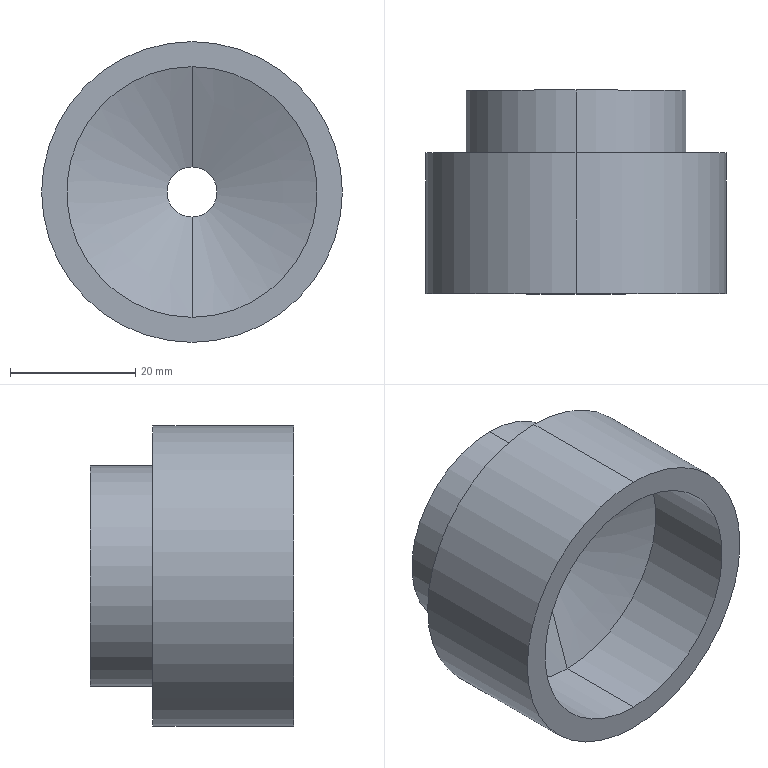Part | SolidWorks | features Revolution 1 | 1 solid | 13 faces | box 48 x 32.5 x 48 mm | volume 28090 mm3 | cylinder 8 | plane 3 | cone 2 | commonest cylinder face diameters 8 x2 35.2 x2 40 x2 48 x2
STEP:
#1=CARTESIAN_POINT('',(0.,0.,24.));
#2=VERTEX_POINT('',#1);
#3=CARTESIAN_POINT('',(0.,0.,-24.));
#4=VERTEX_POINT('',#3);
#5=CARTESIAN_POINT('',(0.,0.,0.));
#6=DIRECTION('',(0.,1.,0.));
#7=DIRECTION('',(0.,0.,1.));
#8=AXIS2_PLACEMENT_3D('',#5,#6,#7);
#9=CIRCLE('',#8,24.);
#10=EDGE_CURVE('',#2,#4,#9,.T.);
#11=ORIENTED_EDGE('',*,*,#10,.T.);
#12=CARTESIAN_POINT('',(0.,22.5,-24.));
#13=VERTEX_POINT('',#12);
#14=CARTESIAN_POINT('',(0.,61.8,-24.));
#15=DIRECTION('',(0.,1.,0.));
#16=VECTOR('',#15,1000.);
#17=LINE('',#14,#16);
#18=EDGE_CURVE('',#4,#13,#17,.T.);
#19=ORIENTED_EDGE('',*,*,#18,.T.);
#20=CARTESIAN_POINT('',(0.,22.5,24.));
#21=VERTEX_POINT('',#20);
#22=CARTESIAN_POINT('',(0.,22.5,0.));
#23=DIRECTION('',(0.,1.,0.));
#24=DIRECTION('',(0.,0.,1.));
#25=AXIS2_PLACEMENT_3D('',#22,#23,#24);
#26=CIRCLE('',#25,24.);
#27=EDGE_CURVE('',#21,#13,#26,.T.);
#28=ORIENTED_EDGE('',*,*,#27,.F.);
#29=CARTESIAN_POINT('',(0.,61.8,24.));
#30=DIRECTION('',(0.,1.,0.));
#31=VECTOR('',#30,1000.);
#32=LINE('',#29,#31);
#33=EDGE_CURVE('',#2,#21,#32,.T.);
#34=ORIENTED_EDGE('',*,*,#33,.F.);
#35=EDGE_LOOP('',(#11,#19,#28,#34));
#36=FACE_OUTER_BOUND('',#35,.T.);
#37=CARTESIAN_POINT('',(0.,61.8,0.));
#38=DIRECTION('',(0.,1.,0.));
#39=DIRECTION('',(0.,0.,1.));
#40=AXIS2_PLACEMENT_3D('',#37,#38,#39);
#41=CYLINDRICAL_SURFACE('',#40,24.);
#42=ADVANCED_FACE('',(#36),#41,.T.);
#43=CARTESIAN_POINT('',(0.,22.5,17.6));
#44=VERTEX_POINT('',#43);
#45=CARTESIAN_POINT('',(0.,22.5,-17.6));
#46=VERTEX_POINT('',#45);
#47=CARTESIAN_POINT('',(0.,22.5,0.));
#48=DIRECTION('',(0.,1.,0.));
#49=DIRECTION('',(0.,0.,1.));
#50=AXIS2_PLACEMENT_3D('',#47,#48,#49);
#51=CIRCLE('',#50,17.6);
#52=EDGE_CURVE('',#44,#46,#51,.T.);
#53=ORIENTED_EDGE('',*,*,#52,.T.);
#54=CARTESIAN_POINT('',(0.,32.5,-17.6));
#55=VERTEX_POINT('',#54);
#56=CARTESIAN_POINT('',(0.,61.8,-17.6));
#57=DIRECTION('',(0.,1.,0.));
#58=VECTOR('',#57,1000.);
#59=LINE('',#56,#58);
#60=EDGE_CURVE('',#46,#55,#59,.T.);
#61=ORIENTED_EDGE('',*,*,#60,.T.);
#62=CARTESIAN_POINT('',(0.,32.5,17.6));
#63=VERTEX_POINT('',#62);
#64=CARTESIAN_POINT('',(0.,32.5,0.));
#65=DIRECTION('',(0.,1.,0.));
#66=DIRECTION('',(0.,0.,1.));
#67=AXIS2_PLACEMENT_3D('',#64,#65,#66);
#68=CIRCLE('',#67,17.6);
#69=EDGE_CURVE('',#63,#55,#68,.T.);
#70=ORIENTED_EDGE('',*,*,#69,.F.);
#71=CARTESIAN_POINT('',(0.,61.8,17.6));
#72=DIRECTION('',(0.,1.,0.));
#73=VECTOR('',#72,1000.);
#74=LINE('',#71,#73);
#75=EDGE_CURVE('',#44,#63,#74,.T.);
#76=ORIENTED_EDGE('',*,*,#75,.F.);
#77=EDGE_LOOP('',(#53,#61,#70,#76));
#78=FACE_OUTER_BOUND('',#77,.T.);
#79=CARTESIAN_POINT('',(0.,61.8,0.));
#80=DIRECTION('',(0.,1.,0.));
#81=DIRECTION('',(0.,0.,1.));
#82=AXIS2_PLACEMENT_3D('',#79,#80,#81);
#83=CYLINDRICAL_SURFACE('',#82,17.6);
#84=ADVANCED_FACE('',(#78),#83,.T.);
#85=CARTESIAN_POINT('',(0.,20.6,-4.));
#86=VERTEX_POINT('',#85);
#87=CARTESIAN_POINT('',(0.,20.6,4.));
#88=VERTEX_POINT('',#87);
#89=CARTESIAN_POINT('',(0.,20.6,0.));
#90=DIRECTION('',(0.,1.,0.));
#91=DIRECTION('',(0.,0.,1.));
#92=AXIS2_PLACEMENT_3D('',#89,#90,#91);
#93=CIRCLE('',#92,4.);
#94=EDGE_CURVE('',#86,#88,#93,.T.);
#95=ORIENTED_EDGE('',*,*,#94,.F.);
#96=CARTESIAN_POINT('',(0.,32.5,-4.));
#97=VERTEX_POINT('',#96);
#98=CARTESIAN_POINT('',(0.,61.8,-4.));
#99=DIRECTION('',(0.,1.,0.));
#100=VECTOR('',#99,1000.);
#101=LINE('',#98,#100);
#102=EDGE_CURVE('',#86,#97,#101,.T.);
#103=ORIENTED_EDGE('',*,*,#102,.T.);
#104=CARTESIAN_POINT('',(0.,32.5,4.));
#105=VERTEX_POINT('',#104);
#106=CARTESIAN_POINT('',(0.,32.5,0.));
#107=DIRECTION('',(0.,1.,0.));
#108=DIRECTION('',(0.,0.,1.));
#109=AXIS2_PLACEMENT_3D('',#106,#107,#108);
#110=CIRCLE('',#109,4.);
#111=EDGE_CURVE('',#97,#105,#110,.T.);
#112=ORIENTED_EDGE('',*,*,#111,.T.);
#113=CARTESIAN_POINT('',(0.,61.8,4.));
#114=DIRECTION('',(0.,1.,0.));
#115=VECTOR('',#114,1000.);
#116=LINE('',#113,#115);
#117=EDGE_CURVE('',#88,#105,#116,.T.);
#118=ORIENTED_EDGE('',*,*,#117,.F.);
#119=EDGE_LOOP('',(#95,#103,#112,#118));
#120=FACE_OUTER_BOUND('',#119,.T.);
#121=CARTESIAN_POINT('',(0.,61.8,0.));
#122=DIRECTION('',(0.,1.,0.));
#123=DIRECTION('',(0.,0.,1.));
#124=AXIS2_PLACEMENT_3D('',#121,#122,#123);
#125=CYLINDRICAL_SURFACE('',#124,4.);
#126=ADVANCED_FACE('',(#120),#125,.F.);
#127=ORIENTED_EDGE('',*,*,#94,.T.);
#128=CARTESIAN_POINT('',(0.,15.,20.));
#129=VERTEX_POINT('',#128);
#130=CARTESIAN_POINT('',(0.,15.,20.));
#131=DIRECTION('',(0.,-0.3304,0.9439));
#132=VECTOR('',#131,1000.);
#133=LINE('',#130,#132);
#134=EDGE_CURVE('',#88,#129,#133,.T.);
#135=ORIENTED_EDGE('',*,*,#134,.T.);
#136=CARTESIAN_POINT('',(0.,15.,-20.));
#137=VERTEX_POINT('',#136);
#138=CARTESIAN_POINT('',(0.,15.,0.));
#139=DIRECTION('',(0.,1.,0.));
#140=DIRECTION('',(0.,0.,1.));
#141=AXIS2_PLACEMENT_3D('',#138,#139,#140);
#142=CIRCLE('',#141,20.);
#143=EDGE_CURVE('',#137,#129,#142,.T.);
#144=ORIENTED_EDGE('',*,*,#143,.F.);
#145=CARTESIAN_POINT('',(0.,15.,-20.));
#146=DIRECTION('',(0.,-0.3304,-0.9439));
#147=VECTOR('',#146,1000.);
#148=LINE('',#145,#147);
#149=EDGE_CURVE('',#86,#137,#148,.T.);
#150=ORIENTED_EDGE('',*,*,#149,.F.);
#151=EDGE_LOOP('',(#127,#135,#144,#150));
#152=FACE_OUTER_BOUND('',#151,.T.);
#153=CARTESIAN_POINT('',(0.,15.,0.));
#154=DIRECTION('',(0.,-1.,0.));
#155=DIRECTION('',(0.,0.,-1.));
#156=AXIS2_PLACEMENT_3D('',#153,#154,#155);
#157=CONICAL_SURFACE('',#156,20.,1.234);
#158=ADVANCED_FACE('',(#152),#157,.F.);
#159=CARTESIAN_POINT('',(0.,0.,-20.));
#160=VERTEX_POINT('',#159);
#161=CARTESIAN_POINT('',(0.,0.,20.));
#162=VERTEX_POINT('',#161);
#163=CARTESIAN_POINT('',(0.,0.,0.));
#164=DIRECTION('',(0.,1.,0.));
#165=DIRECTION('',(0.,0.,1.));
#166=AXIS2_PLACEMENT_3D('',#163,#164,#165);
#167=CIRCLE('',#166,20.);
#168=EDGE_CURVE('',#160,#162,#167,.T.);
#169=ORIENTED_EDGE('',*,*,#168,.F.);
#170=CARTESIAN_POINT('',(0.,61.8,-20.));
#171=DIRECTION('',(0.,1.,0.));
#172=VECTOR('',#171,1000.);
#173=LINE('',#170,#172);
#174=EDGE_CURVE('',#160,#137,#173,.T.);
#175=ORIENTED_EDGE('',*,*,#174,.T.);
#176=ORIENTED_EDGE('',*,*,#143,.T.);
#177=CARTESIAN_POINT('',(0.,61.8,20.));
#178=DIRECTION('',(0.,1.,0.));
#179=VECTOR('',#178,1000.);
#180=LINE('',#177,#179);
#181=EDGE_CURVE('',#162,#129,#180,.T.);
#182=ORIENTED_EDGE('',*,*,#181,.F.);
#183=EDGE_LOOP('',(#169,#175,#176,#182));
#184=FACE_OUTER_BOUND('',#183,.T.);
#185=CARTESIAN_POINT('',(0.,61.8,0.));
#186=DIRECTION('',(0.,1.,0.));
#187=DIRECTION('',(0.,0.,1.));
#188=AXIS2_PLACEMENT_3D('',#185,#186,#187);
#189=CYLINDRICAL_SURFACE('',#188,20.);
#190=ADVANCED_FACE('',(#184),#189,.F.);
#191=ORIENTED_EDGE('',*,*,#174,.F.);
#192=CARTESIAN_POINT('',(0.,0.,0.));
#193=DIRECTION('',(0.,1.,0.));
#194=DIRECTION('',(0.,0.,1.));
#195=AXIS2_PLACEMENT_3D('',#192,#193,#194);
#196=CIRCLE('',#195,20.);
#197=EDGE_CURVE('',#162,#160,#196,.T.);
#198=ORIENTED_EDGE('',*,*,#197,.F.);
#199=ORIENTED_EDGE('',*,*,#181,.T.);
#200=CARTESIAN_POINT('',(0.,15.,0.));
#201=DIRECTION('',(0.,1.,0.));
#202=DIRECTION('',(0.,0.,1.));
#203=AXIS2_PLACEMENT_3D('',#200,#201,#202);
#204=CIRCLE('',#203,20.);
#205=EDGE_CURVE('',#129,#137,#204,.T.);
#206=ORIENTED_EDGE('',*,*,#205,.T.);
#207=EDGE_LOOP('',(#191,#198,#199,#206));
#208=FACE_OUTER_BOUND('',#207,.T.);
#209=CARTESIAN_POINT('',(0.,61.8,0.));
#210=DIRECTION('',(0.,1.,0.));
#211=DIRECTION('',(0.,0.,1.));
#212=AXIS2_PLACEMENT_3D('',#209,#210,#211);
#213=CYLINDRICAL_SURFACE('',#212,20.);
#214=ADVANCED_FACE('',(#208),#213,.F.);
#215=ORIENTED_EDGE('',*,*,#134,.F.);
#216=CARTESIAN_POINT('',(0.,20.6,0.));
#217=DIRECTION('',(0.,1.,0.));
#218=DIRECTION('',(0.,0.,1.));
#219=AXIS2_PLACEMENT_3D('',#216,#217,#218);
#220=CIRCLE('',#219,4.);
#221=EDGE_CURVE('',#88,#86,#220,.T.);
#222=ORIENTED_EDGE('',*,*,#221,.T.);
#223=ORIENTED_EDGE('',*,*,#149,.T.);
#224=ORIENTED_EDGE('',*,*,#205,.F.);
#225=EDGE_LOOP('',(#215,#222,#223,#224));
#226=FACE_OUTER_BOUND('',#225,.T.);
#227=CARTESIAN_POINT('',(0.,15.,0.));
#228=DIRECTION('',(0.,-1.,0.));
#229=DIRECTION('',(0.,0.,-1.));
#230=AXIS2_PLACEMENT_3D('',#227,#228,#229);
#231=CONICAL_SURFACE('',#230,20.,1.234);
#232=ADVANCED_FACE('',(#226),#231,.F.);
#233=ORIENTED_EDGE('',*,*,#102,.F.);
#234=ORIENTED_EDGE('',*,*,#221,.F.);
#235=ORIENTED_EDGE('',*,*,#117,.T.);
#236=CARTESIAN_POINT('',(0.,32.5,0.));
#237=DIRECTION('',(0.,1.,0.));
#238=DIRECTION('',(0.,0.,1.));
#239=AXIS2_PLACEMENT_3D('',#236,#237,#238);
#240=CIRCLE('',#239,4.);
#241=EDGE_CURVE('',#105,#97,#240,.T.);
#242=ORIENTED_EDGE('',*,*,#241,.T.);
#243=EDGE_LOOP('',(#233,#234,#235,#242));
#244=FACE_OUTER_BOUND('',#243,.T.);
#245=CARTESIAN_POINT('',(0.,61.8,0.));
#246=DIRECTION('',(0.,1.,0.));
#247=DIRECTION('',(0.,0.,1.));
#248=AXIS2_PLACEMENT_3D('',#245,#246,#247);
#249=CYLINDRICAL_SURFACE('',#248,4.);
#250=ADVANCED_FACE('',(#244),#249,.F.);
#251=ORIENTED_EDGE('',*,*,#69,.T.);
#252=CARTESIAN_POINT('',(0.,32.5,0.));
#253=DIRECTION('',(0.,1.,0.));
#254=DIRECTION('',(0.,0.,1.));
#255=AXIS2_PLACEMENT_3D('',#252,#253,#254);
#256=CIRCLE('',#255,17.6);
#257=EDGE_CURVE('',#55,#63,#256,.T.);
#258=ORIENTED_EDGE('',*,*,#257,.T.);
#259=EDGE_LOOP('',(#251,#258));
#260=FACE_OUTER_BOUND('',#259,.T.);
#261=ORIENTED_EDGE('',*,*,#241,.F.);
#262=ORIENTED_EDGE('',*,*,#111,.F.);
#263=EDGE_LOOP('',(#261,#262));
#264=FACE_BOUND('',#263,.T.);
#265=CARTESIAN_POINT('',(-4.,32.5,0.));
#266=DIRECTION('',(0.,1.,0.));
#267=DIRECTION('',(0.,0.,1.));
#268=AXIS2_PLACEMENT_3D('',#265,#266,#267);
#269=PLANE('',#268);
#270=ADVANCED_FACE('',(#260,#264),#269,.T.);
#271=ORIENTED_EDGE('',*,*,#60,.F.);
#272=CARTESIAN_POINT('',(0.,22.5,0.));
#273=DIRECTION('',(0.,1.,0.));
#274=DIRECTION('',(0.,0.,1.));
#275=AXIS2_PLACEMENT_3D('',#272,#273,#274);
#276=CIRCLE('',#275,17.6);
#277=EDGE_CURVE('',#46,#44,#276,.T.);
#278=ORIENTED_EDGE('',*,*,#277,.T.);
#279=ORIENTED_EDGE('',*,*,#75,.T.);
#280=ORIENTED_EDGE('',*,*,#257,.F.);
#281=EDGE_LOOP('',(#271,#278,#279,#280));
#282=FACE_OUTER_BOUND('',#281,.T.);
#283=CARTESIAN_POINT('',(0.,61.8,0.));
#284=DIRECTION('',(0.,1.,0.));
#285=DIRECTION('',(0.,0.,1.));
#286=AXIS2_PLACEMENT_3D('',#283,#284,#285);
#287=CYLINDRICAL_SURFACE('',#286,17.6);
#288=ADVANCED_FACE('',(#282),#287,.T.);
#289=ORIENTED_EDGE('',*,*,#27,.T.);
#290=CARTESIAN_POINT('',(0.,22.5,0.));
#291=DIRECTION('',(0.,1.,0.));
#292=DIRECTION('',(0.,0.,1.));
#293=AXIS2_PLACEMENT_3D('',#290,#291,#292);
#294=CIRCLE('',#293,24.);
#295=EDGE_CURVE('',#13,#21,#294,.T.);
#296=ORIENTED_EDGE('',*,*,#295,.T.);
#297=EDGE_LOOP('',(#289,#296));
#298=FACE_OUTER_BOUND('',#297,.T.);
#299=ORIENTED_EDGE('',*,*,#52,.F.);
#300=ORIENTED_EDGE('',*,*,#277,.F.);
#301=EDGE_LOOP('',(#299,#300));
#302=FACE_BOUND('',#301,.T.);
#303=CARTESIAN_POINT('',(-17.6,22.5,0.));
#304=DIRECTION('',(0.,1.,0.));
#305=DIRECTION('',(0.,0.,1.));
#306=AXIS2_PLACEMENT_3D('',#303,#304,#305);
#307=PLANE('',#306);
#308=ADVANCED_FACE('',(#298,#302),#307,.T.);
#309=ORIENTED_EDGE('',*,*,#18,.F.);
#310=CARTESIAN_POINT('',(0.,0.,0.));
#311=DIRECTION('',(0.,1.,0.));
#312=DIRECTION('',(0.,0.,1.));
#313=AXIS2_PLACEMENT_3D('',#310,#311,#312);
#314=CIRCLE('',#313,24.);
#315=EDGE_CURVE('',#4,#2,#314,.T.);
#316=ORIENTED_EDGE('',*,*,#315,.T.);
#317=ORIENTED_EDGE('',*,*,#33,.T.);
#318=ORIENTED_EDGE('',*,*,#295,.F.);
#319=EDGE_LOOP('',(#309,#316,#317,#318));
#320=FACE_OUTER_BOUND('',#319,.T.);
#321=CARTESIAN_POINT('',(0.,61.8,0.));
#322=DIRECTION('',(0.,1.,0.));
#323=DIRECTION('',(0.,0.,1.));
#324=AXIS2_PLACEMENT_3D('',#321,#322,#323);
#325=CYLINDRICAL_SURFACE('',#324,24.);
#326=ADVANCED_FACE('',(#320),#325,.T.);
#327=ORIENTED_EDGE('',*,*,#197,.T.);
#328=ORIENTED_EDGE('',*,*,#168,.T.);
#329=EDGE_LOOP('',(#327,#328));
#330=FACE_BOUND('',#329,.T.);
#331=ORIENTED_EDGE('',*,*,#10,.F.);
#332=ORIENTED_EDGE('',*,*,#315,.F.);
#333=EDGE_LOOP('',(#331,#332));
#334=FACE_OUTER_BOUND('',#333,.T.);
#335=CARTESIAN_POINT('',(-24.,0.,0.));
#336=DIRECTION('',(0.,-1.,0.));
#337=DIRECTION('',(0.,0.,-1.));
#338=AXIS2_PLACEMENT_3D('',#335,#336,#337);
#339=PLANE('',#338);
#340=ADVANCED_FACE('',(#330,#334),#339,.T.);
#341=CLOSED_SHELL('',(#42,#84,#126,#158,#190,#214,#232,#250,#270,#288,#308,#326,#340));
#342=MANIFOLD_SOLID_BREP('',#341);
#343=CARTESIAN_POINT('',(0.,0.,0.));
#344=DIRECTION('',(0.,0.,1.));
#345=DIRECTION('',(1.,0.,0.));
#346=AXIS2_PLACEMENT_3D('',#343,#344,#345);
#347=(LENGTH_UNIT()NAMED_UNIT(*)SI_UNIT(.MILLI.,.METRE.));
#348=UNCERTAINTY_MEASURE_WITH_UNIT(LENGTH_MEASURE(0.00001),#347,'','');
#349=(NAMED_UNIT(*)PLANE_ANGLE_UNIT()SI_UNIT($,.RADIAN.));
#350=(NAMED_UNIT(*)SI_UNIT($,.STERADIAN.)SOLID_ANGLE_UNIT());
#351=(GEOMETRIC_REPRESENTATION_CONTEXT(3)GLOBAL_UNCERTAINTY_ASSIGNED_CONTEXT((#348))GLOBAL_UNIT_ASSIGNED_CONTEXT((#347,#349,#350))REPRESENTATION_CONTEXT('',''));
#352=ADVANCED_BREP_SHAPE_REPRESENTATION('',(#342,#346),#351);